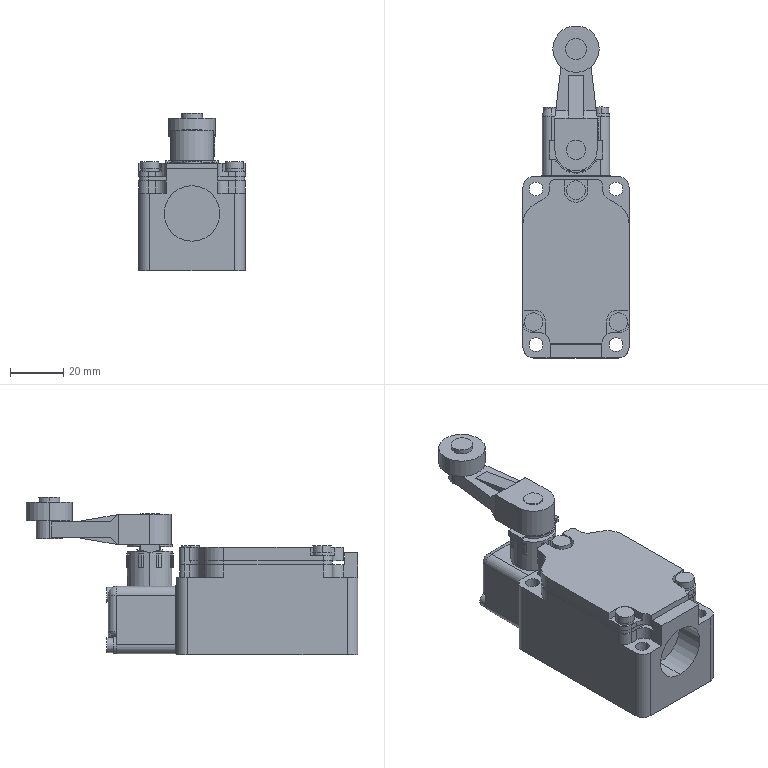Part | SolidWorks | 4 solids | 325 faces | box 40 x 125.15 x 59.4 mm | volume 125288 mm3 | plane 187 | cylinder 130 | torus 8 | commonest cylinder face diameters 8 x18 6 x16 3.5 x12 7 x10 3 x8 5.2 x8